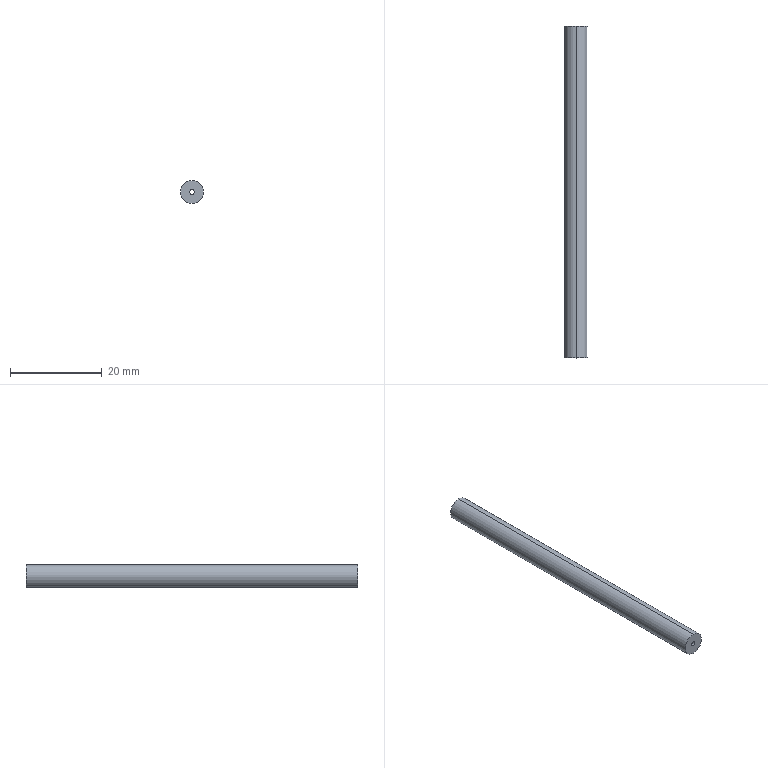Part | SolidWorks | features Extrusion 1, ICE 1, MoveFace 1 | 1 solid | 9 faces | box 5 x 72.2 x 5 mm | volume 919.858 mm3 | cylinder 6 | plane 3 | commonest cylinder face diameters 1 x2 3 x2 5 x2
STEP:
#1=CARTESIAN_POINT('',(0.,-6.7,0.5));
#2=VERTEX_POINT('',#1);
#3=CARTESIAN_POINT('',(0.,-6.7,-0.5));
#4=VERTEX_POINT('',#3);
#5=CARTESIAN_POINT('',(0.,-6.7,0.));
#6=DIRECTION('',(0.,-1.,0.));
#7=DIRECTION('',(0.,0.,-1.));
#8=AXIS2_PLACEMENT_3D('',#5,#6,#7);
#9=CIRCLE('',#8,0.5);
#10=EDGE_CURVE('',#2,#4,#9,.T.);
#11=ORIENTED_EDGE('',*,*,#10,.F.);
#12=CARTESIAN_POINT('',(0.,-8.7,0.5));
#13=VERTEX_POINT('',#12);
#14=CARTESIAN_POINT('',(0.,2.,0.5));
#15=DIRECTION('',(0.,-1.,0.));
#16=VECTOR('',#15,1000.);
#17=LINE('',#14,#16);
#18=EDGE_CURVE('',#2,#13,#17,.T.);
#19=ORIENTED_EDGE('',*,*,#18,.T.);
#20=CARTESIAN_POINT('',(0.,-8.7,-0.5));
#21=VERTEX_POINT('',#20);
#22=CARTESIAN_POINT('',(0.,-8.7,0.));
#23=DIRECTION('',(0.,-1.,0.));
#24=DIRECTION('',(0.,0.,-1.));
#25=AXIS2_PLACEMENT_3D('',#22,#23,#24);
#26=CIRCLE('',#25,0.5);
#27=EDGE_CURVE('',#13,#21,#26,.T.);
#28=ORIENTED_EDGE('',*,*,#27,.T.);
#29=CARTESIAN_POINT('',(0.,2.,-0.5));
#30=DIRECTION('',(0.,-1.,0.));
#31=VECTOR('',#30,1000.);
#32=LINE('',#29,#31);
#33=EDGE_CURVE('',#4,#21,#32,.T.);
#34=ORIENTED_EDGE('',*,*,#33,.F.);
#35=EDGE_LOOP('',(#11,#19,#28,#34));
#36=FACE_OUTER_BOUND('',#35,.T.);
#37=CARTESIAN_POINT('',(0.,2.,0.));
#38=DIRECTION('',(0.,-1.,0.));
#39=DIRECTION('',(0.,0.,-1.));
#40=AXIS2_PLACEMENT_3D('',#37,#38,#39);
#41=CYLINDRICAL_SURFACE('',#40,0.5);
#42=ADVANCED_FACE('',(#36),#41,.F.);
#43=CARTESIAN_POINT('',(0.,63.5,2.5));
#44=VERTEX_POINT('',#43);
#45=CARTESIAN_POINT('',(0.,63.5,-2.5));
#46=VERTEX_POINT('',#45);
#47=CARTESIAN_POINT('',(0.,63.5,0.));
#48=DIRECTION('',(0.,1.,0.));
#49=DIRECTION('',(0.,0.,1.));
#50=AXIS2_PLACEMENT_3D('',#47,#48,#49);
#51=CIRCLE('',#50,2.5);
#52=EDGE_CURVE('',#44,#46,#51,.T.);
#53=ORIENTED_EDGE('',*,*,#52,.F.);
#54=CARTESIAN_POINT('',(0.,-8.7,2.5));
#55=VERTEX_POINT('',#54);
#56=CARTESIAN_POINT('',(0.,63.5,2.5));
#57=DIRECTION('',(0.,-1.,0.));
#58=VECTOR('',#57,1000.);
#59=LINE('',#56,#58);
#60=EDGE_CURVE('',#44,#55,#59,.T.);
#61=ORIENTED_EDGE('',*,*,#60,.T.);
#62=CARTESIAN_POINT('',(0.,-8.7,-2.5));
#63=VERTEX_POINT('',#62);
#64=CARTESIAN_POINT('',(0.,-8.7,0.));
#65=DIRECTION('',(0.,1.,0.));
#66=DIRECTION('',(0.,0.,1.));
#67=AXIS2_PLACEMENT_3D('',#64,#65,#66);
#68=CIRCLE('',#67,2.5);
#69=EDGE_CURVE('',#55,#63,#68,.T.);
#70=ORIENTED_EDGE('',*,*,#69,.T.);
#71=CARTESIAN_POINT('',(0.,63.5,-2.5));
#72=DIRECTION('',(0.,-1.,0.));
#73=VECTOR('',#72,1000.);
#74=LINE('',#71,#73);
#75=EDGE_CURVE('',#46,#63,#74,.T.);
#76=ORIENTED_EDGE('',*,*,#75,.F.);
#77=EDGE_LOOP('',(#53,#61,#70,#76));
#78=FACE_OUTER_BOUND('',#77,.T.);
#79=CARTESIAN_POINT('',(0.,63.5,0.));
#80=DIRECTION('',(0.,-1.,0.));
#81=DIRECTION('',(0.,0.,-1.));
#82=AXIS2_PLACEMENT_3D('',#79,#80,#81);
#83=CYLINDRICAL_SURFACE('',#82,2.5);
#84=ADVANCED_FACE('',(#78),#83,.T.);
#85=CARTESIAN_POINT('',(0.,63.5,-1.5));
#86=VERTEX_POINT('',#85);
#87=CARTESIAN_POINT('',(0.,63.5,1.5));
#88=VERTEX_POINT('',#87);
#89=CARTESIAN_POINT('',(0.,63.5,0.));
#90=DIRECTION('',(0.,1.,0.));
#91=DIRECTION('',(0.,0.,1.));
#92=AXIS2_PLACEMENT_3D('',#89,#90,#91);
#93=CIRCLE('',#92,1.5);
#94=EDGE_CURVE('',#86,#88,#93,.T.);
#95=ORIENTED_EDGE('',*,*,#94,.T.);
#96=CARTESIAN_POINT('',(0.,-6.7,1.5));
#97=VERTEX_POINT('',#96);
#98=CARTESIAN_POINT('',(0.,63.5,1.5));
#99=DIRECTION('',(0.,-1.,0.));
#100=VECTOR('',#99,1000.);
#101=LINE('',#98,#100);
#102=EDGE_CURVE('',#88,#97,#101,.T.);
#103=ORIENTED_EDGE('',*,*,#102,.T.);
#104=CARTESIAN_POINT('',(0.,-6.7,-1.5));
#105=VERTEX_POINT('',#104);
#106=CARTESIAN_POINT('',(0.,-6.7,0.));
#107=DIRECTION('',(0.,-1.,0.));
#108=DIRECTION('',(0.,0.,-1.));
#109=AXIS2_PLACEMENT_3D('',#106,#107,#108);
#110=CIRCLE('',#109,1.5);
#111=EDGE_CURVE('',#97,#105,#110,.T.);
#112=ORIENTED_EDGE('',*,*,#111,.T.);
#113=CARTESIAN_POINT('',(0.,63.5,-1.5));
#114=DIRECTION('',(0.,-1.,0.));
#115=VECTOR('',#114,1000.);
#116=LINE('',#113,#115);
#117=EDGE_CURVE('',#86,#105,#116,.T.);
#118=ORIENTED_EDGE('',*,*,#117,.F.);
#119=EDGE_LOOP('',(#95,#103,#112,#118));
#120=FACE_OUTER_BOUND('',#119,.T.);
#121=CARTESIAN_POINT('',(0.,63.5,0.));
#122=DIRECTION('',(0.,-1.,0.));
#123=DIRECTION('',(0.,0.,-1.));
#124=AXIS2_PLACEMENT_3D('',#121,#122,#123);
#125=CYLINDRICAL_SURFACE('',#124,1.5);
#126=ADVANCED_FACE('',(#120),#125,.F.);
#127=ORIENTED_EDGE('',*,*,#102,.F.);
#128=CARTESIAN_POINT('',(0.,63.5,0.));
#129=DIRECTION('',(0.,1.,0.));
#130=DIRECTION('',(0.,0.,1.));
#131=AXIS2_PLACEMENT_3D('',#128,#129,#130);
#132=CIRCLE('',#131,1.5);
#133=EDGE_CURVE('',#88,#86,#132,.T.);
#134=ORIENTED_EDGE('',*,*,#133,.T.);
#135=ORIENTED_EDGE('',*,*,#117,.T.);
#136=CARTESIAN_POINT('',(0.,-6.7,0.));
#137=DIRECTION('',(0.,-1.,0.));
#138=DIRECTION('',(0.,0.,-1.));
#139=AXIS2_PLACEMENT_3D('',#136,#137,#138);
#140=CIRCLE('',#139,1.5);
#141=EDGE_CURVE('',#105,#97,#140,.T.);
#142=ORIENTED_EDGE('',*,*,#141,.T.);
#143=EDGE_LOOP('',(#127,#134,#135,#142));
#144=FACE_OUTER_BOUND('',#143,.T.);
#145=CARTESIAN_POINT('',(0.,63.5,0.));
#146=DIRECTION('',(0.,-1.,0.));
#147=DIRECTION('',(0.,0.,-1.));
#148=AXIS2_PLACEMENT_3D('',#145,#146,#147);
#149=CYLINDRICAL_SURFACE('',#148,1.5);
#150=ADVANCED_FACE('',(#144),#149,.F.);
#151=CARTESIAN_POINT('',(0.,63.5,0.));
#152=DIRECTION('',(0.,1.,0.));
#153=DIRECTION('',(0.,0.,1.));
#154=AXIS2_PLACEMENT_3D('',#151,#152,#153);
#155=CIRCLE('',#154,2.5);
#156=EDGE_CURVE('',#46,#44,#155,.T.);
#157=ORIENTED_EDGE('',*,*,#156,.T.);
#158=ORIENTED_EDGE('',*,*,#52,.T.);
#159=EDGE_LOOP('',(#157,#158));
#160=FACE_OUTER_BOUND('',#159,.T.);
#161=ORIENTED_EDGE('',*,*,#94,.F.);
#162=ORIENTED_EDGE('',*,*,#133,.F.);
#163=EDGE_LOOP('',(#161,#162));
#164=FACE_BOUND('',#163,.T.);
#165=CARTESIAN_POINT('',(0.,63.5,0.));
#166=DIRECTION('',(0.,1.,0.));
#167=DIRECTION('',(0.,0.,1.));
#168=AXIS2_PLACEMENT_3D('',#165,#166,#167);
#169=PLANE('',#168);
#170=ADVANCED_FACE('',(#160,#164),#169,.T.);
#171=CARTESIAN_POINT('',(0.,-8.7,0.));
#172=DIRECTION('',(0.,1.,0.));
#173=DIRECTION('',(0.,0.,1.));
#174=AXIS2_PLACEMENT_3D('',#171,#172,#173);
#175=CIRCLE('',#174,2.5);
#176=EDGE_CURVE('',#63,#55,#175,.T.);
#177=ORIENTED_EDGE('',*,*,#176,.F.);
#178=ORIENTED_EDGE('',*,*,#69,.F.);
#179=EDGE_LOOP('',(#177,#178));
#180=FACE_OUTER_BOUND('',#179,.T.);
#181=CARTESIAN_POINT('',(0.,-8.7,0.));
#182=DIRECTION('',(0.,-1.,0.));
#183=DIRECTION('',(0.,0.,-1.));
#184=AXIS2_PLACEMENT_3D('',#181,#182,#183);
#185=CIRCLE('',#184,0.5);
#186=EDGE_CURVE('',#21,#13,#185,.T.);
#187=ORIENTED_EDGE('',*,*,#186,.F.);
#188=ORIENTED_EDGE('',*,*,#27,.F.);
#189=EDGE_LOOP('',(#187,#188));
#190=FACE_BOUND('',#189,.T.);
#191=CARTESIAN_POINT('',(0.,-8.7,0.));
#192=DIRECTION('',(0.,1.,0.));
#193=DIRECTION('',(0.,0.,1.));
#194=AXIS2_PLACEMENT_3D('',#191,#192,#193);
#195=PLANE('',#194);
#196=ADVANCED_FACE('',(#180,#190),#195,.F.);
#197=ORIENTED_EDGE('',*,*,#60,.F.);
#198=ORIENTED_EDGE('',*,*,#156,.F.);
#199=ORIENTED_EDGE('',*,*,#75,.T.);
#200=ORIENTED_EDGE('',*,*,#176,.T.);
#201=EDGE_LOOP('',(#197,#198,#199,#200));
#202=FACE_OUTER_BOUND('',#201,.T.);
#203=CARTESIAN_POINT('',(0.,63.5,0.));
#204=DIRECTION('',(0.,-1.,0.));
#205=DIRECTION('',(0.,0.,-1.));
#206=AXIS2_PLACEMENT_3D('',#203,#204,#205);
#207=CYLINDRICAL_SURFACE('',#206,2.5);
#208=ADVANCED_FACE('',(#202),#207,.T.);
#209=CARTESIAN_POINT('',(0.,-6.7,0.));
#210=DIRECTION('',(0.,-1.,0.));
#211=DIRECTION('',(0.,0.,-1.));
#212=AXIS2_PLACEMENT_3D('',#209,#210,#211);
#213=CIRCLE('',#212,0.5);
#214=EDGE_CURVE('',#4,#2,#213,.T.);
#215=ORIENTED_EDGE('',*,*,#214,.T.);
#216=ORIENTED_EDGE('',*,*,#10,.T.);
#217=EDGE_LOOP('',(#215,#216));
#218=FACE_BOUND('',#217,.T.);
#219=ORIENTED_EDGE('',*,*,#141,.F.);
#220=ORIENTED_EDGE('',*,*,#111,.F.);
#221=EDGE_LOOP('',(#219,#220));
#222=FACE_OUTER_BOUND('',#221,.T.);
#223=CARTESIAN_POINT('',(0.,-6.7,0.));
#224=DIRECTION('',(0.,-1.,0.));
#225=DIRECTION('',(0.,0.,-1.));
#226=AXIS2_PLACEMENT_3D('',#223,#224,#225);
#227=PLANE('',#226);
#228=ADVANCED_FACE('',(#218,#222),#227,.F.);
#229=ORIENTED_EDGE('',*,*,#18,.F.);
#230=ORIENTED_EDGE('',*,*,#214,.F.);
#231=ORIENTED_EDGE('',*,*,#33,.T.);
#232=ORIENTED_EDGE('',*,*,#186,.T.);
#233=EDGE_LOOP('',(#229,#230,#231,#232));
#234=FACE_OUTER_BOUND('',#233,.T.);
#235=CARTESIAN_POINT('',(0.,2.,0.));
#236=DIRECTION('',(0.,-1.,0.));
#237=DIRECTION('',(0.,0.,-1.));
#238=AXIS2_PLACEMENT_3D('',#235,#236,#237);
#239=CYLINDRICAL_SURFACE('',#238,0.5);
#240=ADVANCED_FACE('',(#234),#239,.F.);
#241=CLOSED_SHELL('',(#42,#84,#126,#150,#170,#196,#208,#228,#240));
#242=MANIFOLD_SOLID_BREP('',#241);
#243=CARTESIAN_POINT('',(0.,0.,0.));
#244=DIRECTION('',(0.,0.,1.));
#245=DIRECTION('',(1.,0.,0.));
#246=AXIS2_PLACEMENT_3D('',#243,#244,#245);
#247=(LENGTH_UNIT()NAMED_UNIT(*)SI_UNIT(.MILLI.,.METRE.));
#248=UNCERTAINTY_MEASURE_WITH_UNIT(LENGTH_MEASURE(0.00001),#247,'','');
#249=(NAMED_UNIT(*)PLANE_ANGLE_UNIT()SI_UNIT($,.RADIAN.));
#250=(NAMED_UNIT(*)SI_UNIT($,.STERADIAN.)SOLID_ANGLE_UNIT());
#251=(GEOMETRIC_REPRESENTATION_CONTEXT(3)GLOBAL_UNCERTAINTY_ASSIGNED_CONTEXT((#248))GLOBAL_UNIT_ASSIGNED_CONTEXT((#247,#249,#250))REPRESENTATION_CONTEXT('',''));
#252=ADVANCED_BREP_SHAPE_REPRESENTATION('',(#242,#246),#251);